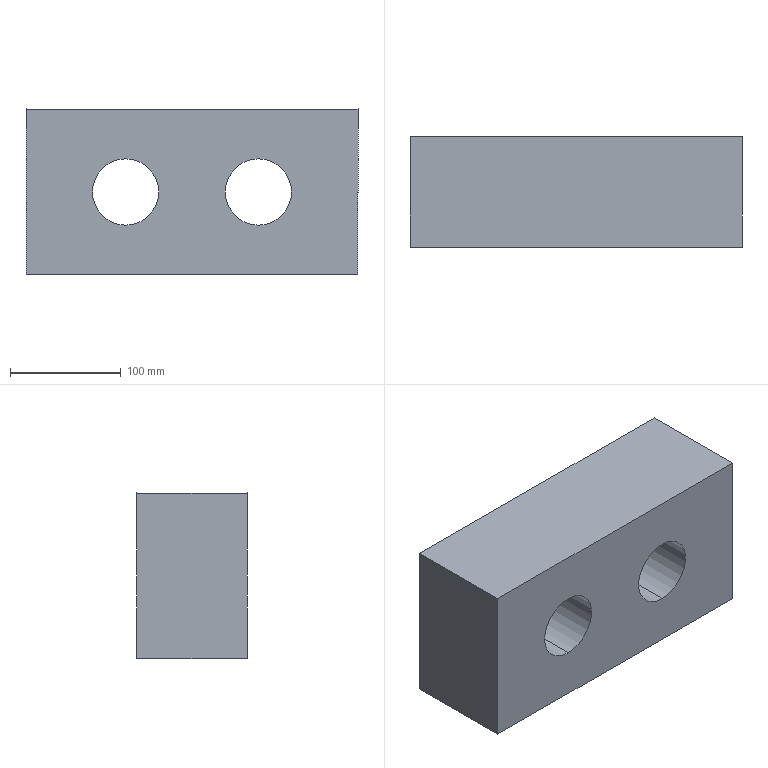Part | SolidWorks | features Extrusion 1 | 1 solid | 10 faces | box 300 x 100 x 150 mm | volume 3934513 mm3 | plane 6 | cylinder 4 | commonest cylinder face diameters 60 x4
STEP:
#1=CARTESIAN_POINT('',(-60.,50.,-30.));
#2=VERTEX_POINT('',#1);
#3=CARTESIAN_POINT('',(-60.,50.,30.));
#4=VERTEX_POINT('',#3);
#5=CARTESIAN_POINT('',(-60.,50.,0.));
#6=DIRECTION('',(0.,1.,0.));
#7=DIRECTION('',(0.,0.,1.));
#8=AXIS2_PLACEMENT_3D('',#5,#6,#7);
#9=CIRCLE('',#8,30.);
#10=EDGE_CURVE('',#2,#4,#9,.T.);
#11=ORIENTED_EDGE('',*,*,#10,.T.);
#12=CARTESIAN_POINT('',(-60.,-50.,30.));
#13=VERTEX_POINT('',#12);
#14=CARTESIAN_POINT('',(-60.,50.,30.));
#15=DIRECTION('',(0.,-1.,0.));
#16=VECTOR('',#15,1000.);
#17=LINE('',#14,#16);
#18=EDGE_CURVE('',#4,#13,#17,.T.);
#19=ORIENTED_EDGE('',*,*,#18,.T.);
#20=CARTESIAN_POINT('',(-60.,-50.,-30.));
#21=VERTEX_POINT('',#20);
#22=CARTESIAN_POINT('',(-60.,-50.,0.));
#23=DIRECTION('',(0.,1.,0.));
#24=DIRECTION('',(0.,0.,1.));
#25=AXIS2_PLACEMENT_3D('',#22,#23,#24);
#26=CIRCLE('',#25,30.);
#27=EDGE_CURVE('',#21,#13,#26,.T.);
#28=ORIENTED_EDGE('',*,*,#27,.F.);
#29=CARTESIAN_POINT('',(-60.,50.,-30.));
#30=DIRECTION('',(0.,-1.,0.));
#31=VECTOR('',#30,1000.);
#32=LINE('',#29,#31);
#33=EDGE_CURVE('',#2,#21,#32,.T.);
#34=ORIENTED_EDGE('',*,*,#33,.F.);
#35=EDGE_LOOP('',(#11,#19,#28,#34));
#36=FACE_OUTER_BOUND('',#35,.T.);
#37=CARTESIAN_POINT('',(-60.,50.,0.));
#38=DIRECTION('',(0.,-1.,0.));
#39=DIRECTION('',(0.,0.,-1.));
#40=AXIS2_PLACEMENT_3D('',#37,#38,#39);
#41=CYLINDRICAL_SURFACE('',#40,30.);
#42=ADVANCED_FACE('',(#36),#41,.F.);
#43=CARTESIAN_POINT('',(60.,50.,-30.));
#44=VERTEX_POINT('',#43);
#45=CARTESIAN_POINT('',(60.,50.,30.));
#46=VERTEX_POINT('',#45);
#47=CARTESIAN_POINT('',(60.,50.,0.));
#48=DIRECTION('',(0.,1.,0.));
#49=DIRECTION('',(0.,0.,1.));
#50=AXIS2_PLACEMENT_3D('',#47,#48,#49);
#51=CIRCLE('',#50,30.);
#52=EDGE_CURVE('',#44,#46,#51,.T.);
#53=ORIENTED_EDGE('',*,*,#52,.T.);
#54=CARTESIAN_POINT('',(60.,-50.,30.));
#55=VERTEX_POINT('',#54);
#56=CARTESIAN_POINT('',(60.,50.,30.));
#57=DIRECTION('',(0.,-1.,0.));
#58=VECTOR('',#57,1000.);
#59=LINE('',#56,#58);
#60=EDGE_CURVE('',#46,#55,#59,.T.);
#61=ORIENTED_EDGE('',*,*,#60,.T.);
#62=CARTESIAN_POINT('',(60.,-50.,-30.));
#63=VERTEX_POINT('',#62);
#64=CARTESIAN_POINT('',(60.,-50.,0.));
#65=DIRECTION('',(0.,1.,0.));
#66=DIRECTION('',(0.,0.,1.));
#67=AXIS2_PLACEMENT_3D('',#64,#65,#66);
#68=CIRCLE('',#67,30.);
#69=EDGE_CURVE('',#63,#55,#68,.T.);
#70=ORIENTED_EDGE('',*,*,#69,.F.);
#71=CARTESIAN_POINT('',(60.,50.,-30.));
#72=DIRECTION('',(0.,-1.,0.));
#73=VECTOR('',#72,1000.);
#74=LINE('',#71,#73);
#75=EDGE_CURVE('',#44,#63,#74,.T.);
#76=ORIENTED_EDGE('',*,*,#75,.F.);
#77=EDGE_LOOP('',(#53,#61,#70,#76));
#78=FACE_OUTER_BOUND('',#77,.T.);
#79=CARTESIAN_POINT('',(60.,50.,0.));
#80=DIRECTION('',(0.,-1.,0.));
#81=DIRECTION('',(0.,0.,-1.));
#82=AXIS2_PLACEMENT_3D('',#79,#80,#81);
#83=CYLINDRICAL_SURFACE('',#82,30.);
#84=ADVANCED_FACE('',(#78),#83,.F.);
#85=ORIENTED_EDGE('',*,*,#52,.F.);
#86=CARTESIAN_POINT('',(60.,50.,0.));
#87=DIRECTION('',(0.,1.,0.));
#88=DIRECTION('',(0.,0.,1.));
#89=AXIS2_PLACEMENT_3D('',#86,#87,#88);
#90=CIRCLE('',#89,30.);
#91=EDGE_CURVE('',#46,#44,#90,.T.);
#92=ORIENTED_EDGE('',*,*,#91,.F.);
#93=EDGE_LOOP('',(#85,#92));
#94=FACE_BOUND('',#93,.T.);
#95=CARTESIAN_POINT('',(150.,50.,75.));
#96=VERTEX_POINT('',#95);
#97=CARTESIAN_POINT('',(150.,50.,-75.));
#98=VERTEX_POINT('',#97);
#99=CARTESIAN_POINT('',(150.,50.,-75.));
#100=DIRECTION('',(0.,0.,-1.));
#101=VECTOR('',#100,1000.);
#102=LINE('',#99,#101);
#103=EDGE_CURVE('',#96,#98,#102,.T.);
#104=ORIENTED_EDGE('',*,*,#103,.T.);
#105=CARTESIAN_POINT('',(-150.,50.,-75.));
#106=VERTEX_POINT('',#105);
#107=CARTESIAN_POINT('',(-150.,50.,-75.));
#108=DIRECTION('',(-1.,0.,0.));
#109=VECTOR('',#108,1000.);
#110=LINE('',#107,#109);
#111=EDGE_CURVE('',#98,#106,#110,.T.);
#112=ORIENTED_EDGE('',*,*,#111,.T.);
#113=CARTESIAN_POINT('',(-150.,50.,75.));
#114=VERTEX_POINT('',#113);
#115=CARTESIAN_POINT('',(-150.,50.,-75.));
#116=DIRECTION('',(0.,0.,1.));
#117=VECTOR('',#116,1000.);
#118=LINE('',#115,#117);
#119=EDGE_CURVE('',#106,#114,#118,.T.);
#120=ORIENTED_EDGE('',*,*,#119,.T.);
#121=CARTESIAN_POINT('',(-150.,50.,75.));
#122=DIRECTION('',(1.,0.,0.));
#123=VECTOR('',#122,1000.);
#124=LINE('',#121,#123);
#125=EDGE_CURVE('',#114,#96,#124,.T.);
#126=ORIENTED_EDGE('',*,*,#125,.T.);
#127=EDGE_LOOP('',(#104,#112,#120,#126));
#128=FACE_OUTER_BOUND('',#127,.T.);
#129=ORIENTED_EDGE('',*,*,#10,.F.);
#130=CARTESIAN_POINT('',(-60.,50.,0.));
#131=DIRECTION('',(0.,1.,0.));
#132=DIRECTION('',(0.,0.,1.));
#133=AXIS2_PLACEMENT_3D('',#130,#131,#132);
#134=CIRCLE('',#133,30.);
#135=EDGE_CURVE('',#4,#2,#134,.T.);
#136=ORIENTED_EDGE('',*,*,#135,.F.);
#137=EDGE_LOOP('',(#129,#136));
#138=FACE_BOUND('',#137,.T.);
#139=CARTESIAN_POINT('',(0.,50.,0.));
#140=DIRECTION('',(0.,1.,0.));
#141=DIRECTION('',(0.,0.,1.));
#142=AXIS2_PLACEMENT_3D('',#139,#140,#141);
#143=PLANE('',#142);
#144=ADVANCED_FACE('',(#94,#128,#138),#143,.T.);
#145=CARTESIAN_POINT('',(150.,-50.,75.));
#146=VERTEX_POINT('',#145);
#147=CARTESIAN_POINT('',(150.,-50.,-75.));
#148=VERTEX_POINT('',#147);
#149=CARTESIAN_POINT('',(150.,-50.,-75.));
#150=DIRECTION('',(0.,0.,-1.));
#151=VECTOR('',#150,1000.);
#152=LINE('',#149,#151);
#153=EDGE_CURVE('',#146,#148,#152,.T.);
#154=ORIENTED_EDGE('',*,*,#153,.F.);
#155=CARTESIAN_POINT('',(-150.,-50.,75.));
#156=VERTEX_POINT('',#155);
#157=CARTESIAN_POINT('',(-150.,-50.,75.));
#158=DIRECTION('',(1.,0.,0.));
#159=VECTOR('',#158,1000.);
#160=LINE('',#157,#159);
#161=EDGE_CURVE('',#156,#146,#160,.T.);
#162=ORIENTED_EDGE('',*,*,#161,.F.);
#163=CARTESIAN_POINT('',(-150.,-50.,-75.));
#164=VERTEX_POINT('',#163);
#165=CARTESIAN_POINT('',(-150.,-50.,-75.));
#166=DIRECTION('',(0.,0.,1.));
#167=VECTOR('',#166,1000.);
#168=LINE('',#165,#167);
#169=EDGE_CURVE('',#164,#156,#168,.T.);
#170=ORIENTED_EDGE('',*,*,#169,.F.);
#171=CARTESIAN_POINT('',(-150.,-50.,-75.));
#172=DIRECTION('',(-1.,0.,0.));
#173=VECTOR('',#172,1000.);
#174=LINE('',#171,#173);
#175=EDGE_CURVE('',#148,#164,#174,.T.);
#176=ORIENTED_EDGE('',*,*,#175,.F.);
#177=EDGE_LOOP('',(#154,#162,#170,#176));
#178=FACE_OUTER_BOUND('',#177,.T.);
#179=ORIENTED_EDGE('',*,*,#69,.T.);
#180=CARTESIAN_POINT('',(60.,-50.,0.));
#181=DIRECTION('',(0.,1.,0.));
#182=DIRECTION('',(0.,0.,1.));
#183=AXIS2_PLACEMENT_3D('',#180,#181,#182);
#184=CIRCLE('',#183,30.);
#185=EDGE_CURVE('',#55,#63,#184,.T.);
#186=ORIENTED_EDGE('',*,*,#185,.T.);
#187=EDGE_LOOP('',(#179,#186));
#188=FACE_BOUND('',#187,.T.);
#189=ORIENTED_EDGE('',*,*,#27,.T.);
#190=CARTESIAN_POINT('',(-60.,-50.,0.));
#191=DIRECTION('',(0.,1.,0.));
#192=DIRECTION('',(0.,0.,1.));
#193=AXIS2_PLACEMENT_3D('',#190,#191,#192);
#194=CIRCLE('',#193,30.);
#195=EDGE_CURVE('',#13,#21,#194,.T.);
#196=ORIENTED_EDGE('',*,*,#195,.T.);
#197=EDGE_LOOP('',(#189,#196));
#198=FACE_BOUND('',#197,.T.);
#199=CARTESIAN_POINT('',(0.,-50.,0.));
#200=DIRECTION('',(0.,1.,0.));
#201=DIRECTION('',(0.,0.,1.));
#202=AXIS2_PLACEMENT_3D('',#199,#200,#201);
#203=PLANE('',#202);
#204=ADVANCED_FACE('',(#178,#188,#198),#203,.F.);
#205=ORIENTED_EDGE('',*,*,#153,.T.);
#206=CARTESIAN_POINT('',(150.,50.,-75.));
#207=DIRECTION('',(0.,-1.,0.));
#208=VECTOR('',#207,1000.);
#209=LINE('',#206,#208);
#210=EDGE_CURVE('',#98,#148,#209,.T.);
#211=ORIENTED_EDGE('',*,*,#210,.F.);
#212=ORIENTED_EDGE('',*,*,#103,.F.);
#213=CARTESIAN_POINT('',(150.,50.,75.));
#214=DIRECTION('',(0.,-1.,0.));
#215=VECTOR('',#214,1000.);
#216=LINE('',#213,#215);
#217=EDGE_CURVE('',#96,#146,#216,.T.);
#218=ORIENTED_EDGE('',*,*,#217,.T.);
#219=EDGE_LOOP('',(#205,#211,#212,#218));
#220=FACE_OUTER_BOUND('',#219,.T.);
#221=CARTESIAN_POINT('',(150.,50.,-75.));
#222=DIRECTION('',(-1.,0.,0.));
#223=DIRECTION('',(0.,0.,1.));
#224=AXIS2_PLACEMENT_3D('',#221,#222,#223);
#225=PLANE('',#224);
#226=ADVANCED_FACE('',(#220),#225,.F.);
#227=ORIENTED_EDGE('',*,*,#175,.T.);
#228=CARTESIAN_POINT('',(-150.,50.,-75.));
#229=DIRECTION('',(0.,-1.,0.));
#230=VECTOR('',#229,1000.);
#231=LINE('',#228,#230);
#232=EDGE_CURVE('',#106,#164,#231,.T.);
#233=ORIENTED_EDGE('',*,*,#232,.F.);
#234=ORIENTED_EDGE('',*,*,#111,.F.);
#235=ORIENTED_EDGE('',*,*,#210,.T.);
#236=EDGE_LOOP('',(#227,#233,#234,#235));
#237=FACE_OUTER_BOUND('',#236,.T.);
#238=CARTESIAN_POINT('',(-150.,50.,-75.));
#239=DIRECTION('',(0.,0.,1.));
#240=DIRECTION('',(1.,0.,0.));
#241=AXIS2_PLACEMENT_3D('',#238,#239,#240);
#242=PLANE('',#241);
#243=ADVANCED_FACE('',(#237),#242,.F.);
#244=ORIENTED_EDGE('',*,*,#169,.T.);
#245=CARTESIAN_POINT('',(-150.,50.,75.));
#246=DIRECTION('',(0.,-1.,0.));
#247=VECTOR('',#246,1000.);
#248=LINE('',#245,#247);
#249=EDGE_CURVE('',#114,#156,#248,.T.);
#250=ORIENTED_EDGE('',*,*,#249,.F.);
#251=ORIENTED_EDGE('',*,*,#119,.F.);
#252=ORIENTED_EDGE('',*,*,#232,.T.);
#253=EDGE_LOOP('',(#244,#250,#251,#252));
#254=FACE_OUTER_BOUND('',#253,.T.);
#255=CARTESIAN_POINT('',(-150.,50.,-75.));
#256=DIRECTION('',(1.,0.,0.));
#257=DIRECTION('',(0.,0.,-1.));
#258=AXIS2_PLACEMENT_3D('',#255,#256,#257);
#259=PLANE('',#258);
#260=ADVANCED_FACE('',(#254),#259,.F.);
#261=ORIENTED_EDGE('',*,*,#161,.T.);
#262=ORIENTED_EDGE('',*,*,#217,.F.);
#263=ORIENTED_EDGE('',*,*,#125,.F.);
#264=ORIENTED_EDGE('',*,*,#249,.T.);
#265=EDGE_LOOP('',(#261,#262,#263,#264));
#266=FACE_OUTER_BOUND('',#265,.T.);
#267=CARTESIAN_POINT('',(-150.,50.,75.));
#268=DIRECTION('',(0.,0.,-1.));
#269=DIRECTION('',(-1.,0.,0.));
#270=AXIS2_PLACEMENT_3D('',#267,#268,#269);
#271=PLANE('',#270);
#272=ADVANCED_FACE('',(#266),#271,.F.);
#273=ORIENTED_EDGE('',*,*,#60,.F.);
#274=ORIENTED_EDGE('',*,*,#91,.T.);
#275=ORIENTED_EDGE('',*,*,#75,.T.);
#276=ORIENTED_EDGE('',*,*,#185,.F.);
#277=EDGE_LOOP('',(#273,#274,#275,#276));
#278=FACE_OUTER_BOUND('',#277,.T.);
#279=CARTESIAN_POINT('',(60.,50.,0.));
#280=DIRECTION('',(0.,-1.,0.));
#281=DIRECTION('',(0.,0.,-1.));
#282=AXIS2_PLACEMENT_3D('',#279,#280,#281);
#283=CYLINDRICAL_SURFACE('',#282,30.);
#284=ADVANCED_FACE('',(#278),#283,.F.);
#285=ORIENTED_EDGE('',*,*,#18,.F.);
#286=ORIENTED_EDGE('',*,*,#135,.T.);
#287=ORIENTED_EDGE('',*,*,#33,.T.);
#288=ORIENTED_EDGE('',*,*,#195,.F.);
#289=EDGE_LOOP('',(#285,#286,#287,#288));
#290=FACE_OUTER_BOUND('',#289,.T.);
#291=CARTESIAN_POINT('',(-60.,50.,0.));
#292=DIRECTION('',(0.,-1.,0.));
#293=DIRECTION('',(0.,0.,-1.));
#294=AXIS2_PLACEMENT_3D('',#291,#292,#293);
#295=CYLINDRICAL_SURFACE('',#294,30.);
#296=ADVANCED_FACE('',(#290),#295,.F.);
#297=CLOSED_SHELL('',(#42,#84,#144,#204,#226,#243,#260,#272,#284,#296));
#298=MANIFOLD_SOLID_BREP('',#297);
#299=CARTESIAN_POINT('',(0.,0.,0.));
#300=DIRECTION('',(0.,0.,1.));
#301=DIRECTION('',(1.,0.,0.));
#302=AXIS2_PLACEMENT_3D('',#299,#300,#301);
#303=(LENGTH_UNIT()NAMED_UNIT(*)SI_UNIT(.MILLI.,.METRE.));
#304=UNCERTAINTY_MEASURE_WITH_UNIT(LENGTH_MEASURE(0.00001),#303,'','');
#305=(NAMED_UNIT(*)PLANE_ANGLE_UNIT()SI_UNIT($,.RADIAN.));
#306=(NAMED_UNIT(*)SI_UNIT($,.STERADIAN.)SOLID_ANGLE_UNIT());
#307=(GEOMETRIC_REPRESENTATION_CONTEXT(3)GLOBAL_UNCERTAINTY_ASSIGNED_CONTEXT((#304))GLOBAL_UNIT_ASSIGNED_CONTEXT((#303,#305,#306))REPRESENTATION_CONTEXT('',''));
#308=ADVANCED_BREP_SHAPE_REPRESENTATION('',(#298,#302),#307);